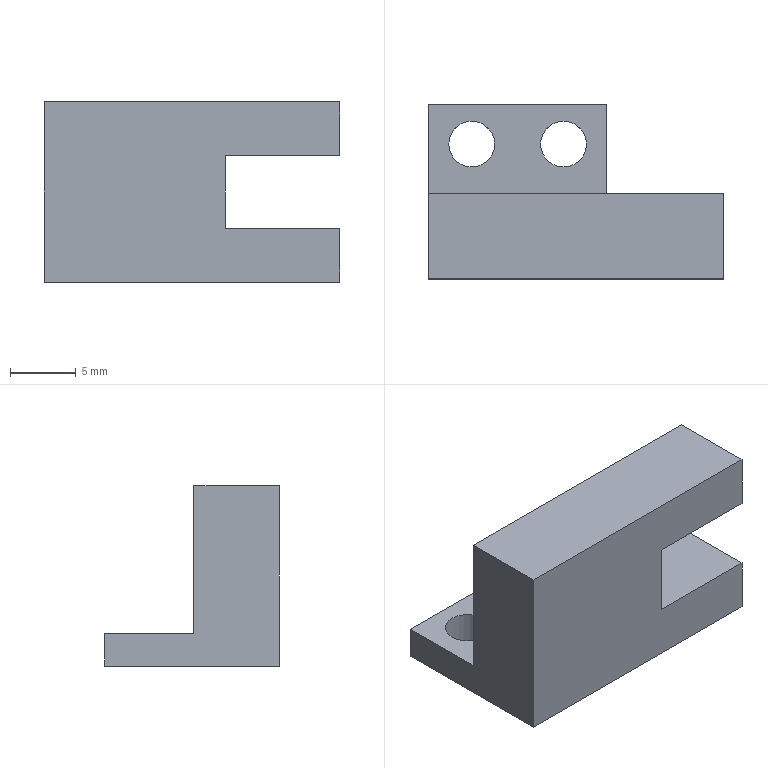Part | STEP file | PM-F54 | 1 solid | 17 faces | box 22.5 x 13.3 x 13.75 mm | volume 1880 mm3 | plane 13 | cylinder 4 | commonest cylinder face diameters 3.5 x4
STEP:
#1=CARTESIAN_POINT('',(5.05,10.3,2.5));
#2=VERTEX_POINT('',#1);
#3=CARTESIAN_POINT('',(1.55,10.3,2.5));
#4=VERTEX_POINT('',#3);
#5=CARTESIAN_POINT('',(3.3,10.3,2.5));
#6=DIRECTION('',(0.,0.,-1.));
#7=DIRECTION('',(-1.,0.,0.));
#8=AXIS2_PLACEMENT_3D('',#5,#6,#7);
#9=CIRCLE('',#8,1.75);
#10=EDGE_CURVE('',#2,#4,#9,.T.);
#11=ORIENTED_EDGE('',*,*,#10,.F.);
#12=CARTESIAN_POINT('',(5.05,10.3,0.));
#13=VERTEX_POINT('',#12);
#14=CARTESIAN_POINT('',(5.05,10.3,2.5));
#15=DIRECTION('',(0.,0.,-1.));
#16=VECTOR('',#15,1000.);
#17=LINE('',#14,#16);
#18=EDGE_CURVE('',#2,#13,#17,.T.);
#19=ORIENTED_EDGE('',*,*,#18,.T.);
#20=CARTESIAN_POINT('',(1.55,10.3,0.));
#21=VERTEX_POINT('',#20);
#22=CARTESIAN_POINT('',(3.3,10.3,0.));
#23=DIRECTION('',(0.,0.,-1.));
#24=DIRECTION('',(-1.,0.,0.));
#25=AXIS2_PLACEMENT_3D('',#22,#23,#24);
#26=CIRCLE('',#25,1.75);
#27=EDGE_CURVE('',#13,#21,#26,.T.);
#28=ORIENTED_EDGE('',*,*,#27,.T.);
#29=CARTESIAN_POINT('',(1.55,10.3,2.5));
#30=DIRECTION('',(0.,0.,-1.));
#31=VECTOR('',#30,1000.);
#32=LINE('',#29,#31);
#33=EDGE_CURVE('',#4,#21,#32,.T.);
#34=ORIENTED_EDGE('',*,*,#33,.F.);
#35=EDGE_LOOP('',(#11,#19,#28,#34));
#36=FACE_OUTER_BOUND('',#35,.T.);
#37=CARTESIAN_POINT('',(3.3,10.3,2.5));
#38=DIRECTION('',(0.,0.,-1.));
#39=DIRECTION('',(-1.,0.,0.));
#40=AXIS2_PLACEMENT_3D('',#37,#38,#39);
#41=CYLINDRICAL_SURFACE('',#40,1.75);
#42=ADVANCED_FACE('',(#36),#41,.F.);
#43=CARTESIAN_POINT('',(12.05,10.3,2.5));
#44=VERTEX_POINT('',#43);
#45=CARTESIAN_POINT('',(8.55,10.3,2.5));
#46=VERTEX_POINT('',#45);
#47=CARTESIAN_POINT('',(10.3,10.3,2.5));
#48=DIRECTION('',(0.,0.,-1.));
#49=DIRECTION('',(-1.,0.,0.));
#50=AXIS2_PLACEMENT_3D('',#47,#48,#49);
#51=CIRCLE('',#50,1.75);
#52=EDGE_CURVE('',#44,#46,#51,.T.);
#53=ORIENTED_EDGE('',*,*,#52,.F.);
#54=CARTESIAN_POINT('',(12.05,10.3,0.));
#55=VERTEX_POINT('',#54);
#56=CARTESIAN_POINT('',(12.05,10.3,2.5));
#57=DIRECTION('',(0.,0.,-1.));
#58=VECTOR('',#57,1000.);
#59=LINE('',#56,#58);
#60=EDGE_CURVE('',#44,#55,#59,.T.);
#61=ORIENTED_EDGE('',*,*,#60,.T.);
#62=CARTESIAN_POINT('',(8.55,10.3,0.));
#63=VERTEX_POINT('',#62);
#64=CARTESIAN_POINT('',(10.3,10.3,0.));
#65=DIRECTION('',(0.,0.,-1.));
#66=DIRECTION('',(-1.,0.,0.));
#67=AXIS2_PLACEMENT_3D('',#64,#65,#66);
#68=CIRCLE('',#67,1.75);
#69=EDGE_CURVE('',#55,#63,#68,.T.);
#70=ORIENTED_EDGE('',*,*,#69,.T.);
#71=CARTESIAN_POINT('',(8.55,10.3,2.5));
#72=DIRECTION('',(0.,0.,-1.));
#73=VECTOR('',#72,1000.);
#74=LINE('',#71,#73);
#75=EDGE_CURVE('',#46,#63,#74,.T.);
#76=ORIENTED_EDGE('',*,*,#75,.F.);
#77=EDGE_LOOP('',(#53,#61,#70,#76));
#78=FACE_OUTER_BOUND('',#77,.T.);
#79=CARTESIAN_POINT('',(10.3,10.3,2.5));
#80=DIRECTION('',(0.,0.,-1.));
#81=DIRECTION('',(-1.,0.,0.));
#82=AXIS2_PLACEMENT_3D('',#79,#80,#81);
#83=CYLINDRICAL_SURFACE('',#82,1.75);
#84=ADVANCED_FACE('',(#78),#83,.F.);
#85=CARTESIAN_POINT('',(13.6,6.5,2.5));
#86=VERTEX_POINT('',#85);
#87=CARTESIAN_POINT('',(13.6,6.5,0.));
#88=VERTEX_POINT('',#87);
#89=CARTESIAN_POINT('',(13.6,6.5,2.5));
#90=DIRECTION('',(0.,0.,-1.));
#91=VECTOR('',#90,1000.);
#92=LINE('',#89,#91);
#93=EDGE_CURVE('',#86,#88,#92,.T.);
#94=ORIENTED_EDGE('',*,*,#93,.F.);
#95=CARTESIAN_POINT('',(0.,6.5,2.5));
#96=VERTEX_POINT('',#95);
#97=CARTESIAN_POINT('',(0.,6.5,2.5));
#98=DIRECTION('',(-1.,0.,0.));
#99=VECTOR('',#98,1000.);
#100=LINE('',#97,#99);
#101=EDGE_CURVE('',#86,#96,#100,.T.);
#102=ORIENTED_EDGE('',*,*,#101,.T.);
#103=CARTESIAN_POINT('',(0.,6.5,13.75));
#104=VERTEX_POINT('',#103);
#105=CARTESIAN_POINT('',(0.,6.5,13.75));
#106=DIRECTION('',(0.,0.,-1.));
#107=VECTOR('',#106,1000.);
#108=LINE('',#105,#107);
#109=EDGE_CURVE('',#104,#96,#108,.T.);
#110=ORIENTED_EDGE('',*,*,#109,.F.);
#111=CARTESIAN_POINT('',(22.5,6.5,13.75));
#112=VERTEX_POINT('',#111);
#113=CARTESIAN_POINT('',(0.,6.5,13.75));
#114=DIRECTION('',(-1.,0.,0.));
#115=VECTOR('',#114,1000.);
#116=LINE('',#113,#115);
#117=EDGE_CURVE('',#112,#104,#116,.T.);
#118=ORIENTED_EDGE('',*,*,#117,.F.);
#119=CARTESIAN_POINT('',(22.5,6.5,9.65));
#120=VERTEX_POINT('',#119);
#121=CARTESIAN_POINT('',(22.5,6.5,13.75));
#122=DIRECTION('',(0.,0.,-1.));
#123=VECTOR('',#122,1000.);
#124=LINE('',#121,#123);
#125=EDGE_CURVE('',#112,#120,#124,.T.);
#126=ORIENTED_EDGE('',*,*,#125,.T.);
#127=CARTESIAN_POINT('',(13.8,6.5,9.65));
#128=VERTEX_POINT('',#127);
#129=CARTESIAN_POINT('',(0.,6.5,9.65));
#130=DIRECTION('',(-1.,0.,0.));
#131=VECTOR('',#130,1000.);
#132=LINE('',#129,#131);
#133=EDGE_CURVE('',#120,#128,#132,.T.);
#134=ORIENTED_EDGE('',*,*,#133,.T.);
#135=CARTESIAN_POINT('',(13.8,6.5,4.1));
#136=VERTEX_POINT('',#135);
#137=CARTESIAN_POINT('',(13.8,6.5,9.65));
#138=DIRECTION('',(0.,0.,-1.));
#139=VECTOR('',#138,1000.);
#140=LINE('',#137,#139);
#141=EDGE_CURVE('',#128,#136,#140,.T.);
#142=ORIENTED_EDGE('',*,*,#141,.T.);
#143=CARTESIAN_POINT('',(22.5,6.5,4.1));
#144=VERTEX_POINT('',#143);
#145=CARTESIAN_POINT('',(13.8,6.5,4.1));
#146=DIRECTION('',(1.,0.,0.));
#147=VECTOR('',#146,1000.);
#148=LINE('',#145,#147);
#149=EDGE_CURVE('',#136,#144,#148,.T.);
#150=ORIENTED_EDGE('',*,*,#149,.T.);
#151=CARTESIAN_POINT('',(22.5,6.5,0.));
#152=VERTEX_POINT('',#151);
#153=CARTESIAN_POINT('',(22.5,6.5,13.75));
#154=DIRECTION('',(0.,0.,-1.));
#155=VECTOR('',#154,1000.);
#156=LINE('',#153,#155);
#157=EDGE_CURVE('',#144,#152,#156,.T.);
#158=ORIENTED_EDGE('',*,*,#157,.T.);
#159=CARTESIAN_POINT('',(0.,6.5,0.));
#160=DIRECTION('',(-1.,0.,0.));
#161=VECTOR('',#160,1000.);
#162=LINE('',#159,#161);
#163=EDGE_CURVE('',#152,#88,#162,.T.);
#164=ORIENTED_EDGE('',*,*,#163,.T.);
#165=EDGE_LOOP('',(#94,#102,#110,#118,#126,#134,#142,#150,#158,#164));
#166=FACE_OUTER_BOUND('',#165,.T.);
#167=CARTESIAN_POINT('',(0.,6.5,13.75));
#168=DIRECTION('',(0.,-1.,0.));
#169=DIRECTION('',(0.,0.,-1.));
#170=AXIS2_PLACEMENT_3D('',#167,#168,#169);
#171=PLANE('',#170);
#172=ADVANCED_FACE('',(#166),#171,.F.);
#173=CARTESIAN_POINT('',(22.5,0.,13.75));
#174=VERTEX_POINT('',#173);
#175=CARTESIAN_POINT('',(22.5,0.,9.65));
#176=VERTEX_POINT('',#175);
#177=CARTESIAN_POINT('',(22.5,0.,13.75));
#178=DIRECTION('',(0.,0.,-1.));
#179=VECTOR('',#178,1000.);
#180=LINE('',#177,#179);
#181=EDGE_CURVE('',#174,#176,#180,.T.);
#182=ORIENTED_EDGE('',*,*,#181,.T.);
#183=CARTESIAN_POINT('',(22.5,0.,9.65));
#184=DIRECTION('',(0.,1.,0.));
#185=VECTOR('',#184,1000.);
#186=LINE('',#183,#185);
#187=EDGE_CURVE('',#176,#120,#186,.T.);
#188=ORIENTED_EDGE('',*,*,#187,.T.);
#189=ORIENTED_EDGE('',*,*,#125,.F.);
#190=CARTESIAN_POINT('',(22.5,0.,13.75));
#191=DIRECTION('',(0.,1.,0.));
#192=VECTOR('',#191,1000.);
#193=LINE('',#190,#192);
#194=EDGE_CURVE('',#174,#112,#193,.T.);
#195=ORIENTED_EDGE('',*,*,#194,.F.);
#196=EDGE_LOOP('',(#182,#188,#189,#195));
#197=FACE_OUTER_BOUND('',#196,.T.);
#198=CARTESIAN_POINT('',(22.5,0.,13.75));
#199=DIRECTION('',(-1.,0.,0.));
#200=DIRECTION('',(0.,0.,1.));
#201=AXIS2_PLACEMENT_3D('',#198,#199,#200);
#202=PLANE('',#201);
#203=ADVANCED_FACE('',(#197),#202,.F.);
#204=CARTESIAN_POINT('',(0.,13.3,0.));
#205=VERTEX_POINT('',#204);
#206=CARTESIAN_POINT('',(0.,0.,0.));
#207=VERTEX_POINT('',#206);
#208=CARTESIAN_POINT('',(0.,0.,0.));
#209=DIRECTION('',(0.,-1.,0.));
#210=VECTOR('',#209,1000.);
#211=LINE('',#208,#210);
#212=EDGE_CURVE('',#205,#207,#211,.T.);
#213=ORIENTED_EDGE('',*,*,#212,.T.);
#214=CARTESIAN_POINT('',(0.,0.,13.75));
#215=VERTEX_POINT('',#214);
#216=CARTESIAN_POINT('',(0.,0.,13.75));
#217=DIRECTION('',(0.,0.,-1.));
#218=VECTOR('',#217,1000.);
#219=LINE('',#216,#218);
#220=EDGE_CURVE('',#215,#207,#219,.T.);
#221=ORIENTED_EDGE('',*,*,#220,.F.);
#222=CARTESIAN_POINT('',(0.,0.,13.75));
#223=DIRECTION('',(0.,-1.,0.));
#224=VECTOR('',#223,1000.);
#225=LINE('',#222,#224);
#226=EDGE_CURVE('',#104,#215,#225,.T.);
#227=ORIENTED_EDGE('',*,*,#226,.F.);
#228=ORIENTED_EDGE('',*,*,#109,.T.);
#229=CARTESIAN_POINT('',(0.,13.3,2.5));
#230=VERTEX_POINT('',#229);
#231=CARTESIAN_POINT('',(0.,6.5,2.5));
#232=DIRECTION('',(0.,1.,0.));
#233=VECTOR('',#232,1000.);
#234=LINE('',#231,#233);
#235=EDGE_CURVE('',#96,#230,#234,.T.);
#236=ORIENTED_EDGE('',*,*,#235,.T.);
#237=CARTESIAN_POINT('',(0.,13.3,2.5));
#238=DIRECTION('',(0.,0.,-1.));
#239=VECTOR('',#238,1000.);
#240=LINE('',#237,#239);
#241=EDGE_CURVE('',#230,#205,#240,.T.);
#242=ORIENTED_EDGE('',*,*,#241,.T.);
#243=EDGE_LOOP('',(#213,#221,#227,#228,#236,#242));
#244=FACE_OUTER_BOUND('',#243,.T.);
#245=CARTESIAN_POINT('',(0.,0.,13.75));
#246=DIRECTION('',(1.,0.,0.));
#247=DIRECTION('',(0.,0.,-1.));
#248=AXIS2_PLACEMENT_3D('',#245,#246,#247);
#249=PLANE('',#248);
#250=ADVANCED_FACE('',(#244),#249,.F.);
#251=CARTESIAN_POINT('',(13.8,0.,9.65));
#252=VERTEX_POINT('',#251);
#253=CARTESIAN_POINT('',(13.8,0.,4.1));
#254=VERTEX_POINT('',#253);
#255=CARTESIAN_POINT('',(13.8,0.,9.65));
#256=DIRECTION('',(0.,0.,-1.));
#257=VECTOR('',#256,1000.);
#258=LINE('',#255,#257);
#259=EDGE_CURVE('',#252,#254,#258,.T.);
#260=ORIENTED_EDGE('',*,*,#259,.F.);
#261=CARTESIAN_POINT('',(13.8,0.,9.65));
#262=DIRECTION('',(-1.,0.,0.));
#263=VECTOR('',#262,1000.);
#264=LINE('',#261,#263);
#265=EDGE_CURVE('',#176,#252,#264,.T.);
#266=ORIENTED_EDGE('',*,*,#265,.F.);
#267=ORIENTED_EDGE('',*,*,#181,.F.);
#268=CARTESIAN_POINT('',(0.,0.,13.75));
#269=DIRECTION('',(1.,0.,0.));
#270=VECTOR('',#269,1000.);
#271=LINE('',#268,#270);
#272=EDGE_CURVE('',#215,#174,#271,.T.);
#273=ORIENTED_EDGE('',*,*,#272,.F.);
#274=ORIENTED_EDGE('',*,*,#220,.T.);
#275=CARTESIAN_POINT('',(22.5,0.,0.));
#276=VERTEX_POINT('',#275);
#277=CARTESIAN_POINT('',(0.,0.,0.));
#278=DIRECTION('',(1.,0.,0.));
#279=VECTOR('',#278,1000.);
#280=LINE('',#277,#279);
#281=EDGE_CURVE('',#207,#276,#280,.T.);
#282=ORIENTED_EDGE('',*,*,#281,.T.);
#283=CARTESIAN_POINT('',(22.5,0.,4.1));
#284=VERTEX_POINT('',#283);
#285=CARTESIAN_POINT('',(22.5,0.,13.75));
#286=DIRECTION('',(0.,0.,-1.));
#287=VECTOR('',#286,1000.);
#288=LINE('',#285,#287);
#289=EDGE_CURVE('',#284,#276,#288,.T.);
#290=ORIENTED_EDGE('',*,*,#289,.F.);
#291=CARTESIAN_POINT('',(13.8,0.,4.1));
#292=DIRECTION('',(1.,0.,0.));
#293=VECTOR('',#292,1000.);
#294=LINE('',#291,#293);
#295=EDGE_CURVE('',#254,#284,#294,.T.);
#296=ORIENTED_EDGE('',*,*,#295,.F.);
#297=EDGE_LOOP('',(#260,#266,#267,#273,#274,#282,#290,#296));
#298=FACE_OUTER_BOUND('',#297,.T.);
#299=CARTESIAN_POINT('',(0.,0.,13.75));
#300=DIRECTION('',(0.,1.,0.));
#301=DIRECTION('',(0.,0.,1.));
#302=AXIS2_PLACEMENT_3D('',#299,#300,#301);
#303=PLANE('',#302);
#304=ADVANCED_FACE('',(#298),#303,.F.);
#305=ORIENTED_EDGE('',*,*,#157,.F.);
#306=CARTESIAN_POINT('',(22.5,0.,4.1));
#307=DIRECTION('',(0.,-1.,0.));
#308=VECTOR('',#307,1000.);
#309=LINE('',#306,#308);
#310=EDGE_CURVE('',#144,#284,#309,.T.);
#311=ORIENTED_EDGE('',*,*,#310,.T.);
#312=ORIENTED_EDGE('',*,*,#289,.T.);
#313=CARTESIAN_POINT('',(22.5,0.,0.));
#314=DIRECTION('',(0.,1.,0.));
#315=VECTOR('',#314,1000.);
#316=LINE('',#313,#315);
#317=EDGE_CURVE('',#276,#152,#316,.T.);
#318=ORIENTED_EDGE('',*,*,#317,.T.);
#319=EDGE_LOOP('',(#305,#311,#312,#318));
#320=FACE_OUTER_BOUND('',#319,.T.);
#321=CARTESIAN_POINT('',(22.5,0.,13.75));
#322=DIRECTION('',(-1.,0.,0.));
#323=DIRECTION('',(0.,0.,1.));
#324=AXIS2_PLACEMENT_3D('',#321,#322,#323);
#325=PLANE('',#324);
#326=ADVANCED_FACE('',(#320),#325,.F.);
#327=ORIENTED_EDGE('',*,*,#226,.T.);
#328=ORIENTED_EDGE('',*,*,#272,.T.);
#329=ORIENTED_EDGE('',*,*,#194,.T.);
#330=ORIENTED_EDGE('',*,*,#117,.T.);
#331=EDGE_LOOP('',(#327,#328,#329,#330));
#332=FACE_OUTER_BOUND('',#331,.T.);
#333=CARTESIAN_POINT('',(0.,6.5,13.75));
#334=DIRECTION('',(0.,0.,-1.));
#335=DIRECTION('',(-1.,0.,0.));
#336=AXIS2_PLACEMENT_3D('',#333,#334,#335);
#337=PLANE('',#336);
#338=ADVANCED_FACE('',(#332),#337,.F.);
#339=ORIENTED_EDGE('',*,*,#212,.F.);
#340=CARTESIAN_POINT('',(13.6,13.3,0.));
#341=VERTEX_POINT('',#340);
#342=CARTESIAN_POINT('',(0.,13.3,0.));
#343=DIRECTION('',(1.,0.,0.));
#344=VECTOR('',#343,1000.);
#345=LINE('',#342,#344);
#346=EDGE_CURVE('',#205,#341,#345,.T.);
#347=ORIENTED_EDGE('',*,*,#346,.T.);
#348=CARTESIAN_POINT('',(13.6,6.5,0.));
#349=DIRECTION('',(0.,-1.,0.));
#350=VECTOR('',#349,1000.);
#351=LINE('',#348,#350);
#352=EDGE_CURVE('',#341,#88,#351,.T.);
#353=ORIENTED_EDGE('',*,*,#352,.T.);
#354=ORIENTED_EDGE('',*,*,#163,.F.);
#355=ORIENTED_EDGE('',*,*,#317,.F.);
#356=ORIENTED_EDGE('',*,*,#281,.F.);
#357=EDGE_LOOP('',(#339,#347,#353,#354,#355,#356));
#358=FACE_OUTER_BOUND('',#357,.T.);
#359=CARTESIAN_POINT('',(3.3,10.3,0.));
#360=DIRECTION('',(0.,0.,-1.));
#361=DIRECTION('',(-1.,0.,0.));
#362=AXIS2_PLACEMENT_3D('',#359,#360,#361);
#363=CIRCLE('',#362,1.75);
#364=EDGE_CURVE('',#21,#13,#363,.T.);
#365=ORIENTED_EDGE('',*,*,#364,.F.);
#366=ORIENTED_EDGE('',*,*,#27,.F.);
#367=EDGE_LOOP('',(#365,#366));
#368=FACE_BOUND('',#367,.T.);
#369=CARTESIAN_POINT('',(10.3,10.3,0.));
#370=DIRECTION('',(0.,0.,-1.));
#371=DIRECTION('',(-1.,0.,0.));
#372=AXIS2_PLACEMENT_3D('',#369,#370,#371);
#373=CIRCLE('',#372,1.75);
#374=EDGE_CURVE('',#63,#55,#373,.T.);
#375=ORIENTED_EDGE('',*,*,#374,.F.);
#376=ORIENTED_EDGE('',*,*,#69,.F.);
#377=EDGE_LOOP('',(#375,#376));
#378=FACE_BOUND('',#377,.T.);
#379=CARTESIAN_POINT('',(0.,6.5,0.));
#380=DIRECTION('',(0.,0.,-1.));
#381=DIRECTION('',(-1.,0.,0.));
#382=AXIS2_PLACEMENT_3D('',#379,#380,#381);
#383=PLANE('',#382);
#384=ADVANCED_FACE('',(#358,#368,#378),#383,.T.);
#385=ORIENTED_EDGE('',*,*,#265,.T.);
#386=CARTESIAN_POINT('',(13.8,6.5,9.65));
#387=DIRECTION('',(0.,-1.,0.));
#388=VECTOR('',#387,1000.);
#389=LINE('',#386,#388);
#390=EDGE_CURVE('',#128,#252,#389,.T.);
#391=ORIENTED_EDGE('',*,*,#390,.F.);
#392=ORIENTED_EDGE('',*,*,#133,.F.);
#393=ORIENTED_EDGE('',*,*,#187,.F.);
#394=EDGE_LOOP('',(#385,#391,#392,#393));
#395=FACE_OUTER_BOUND('',#394,.T.);
#396=CARTESIAN_POINT('',(13.8,6.5,9.65));
#397=DIRECTION('',(0.,0.,1.));
#398=DIRECTION('',(1.,0.,0.));
#399=AXIS2_PLACEMENT_3D('',#396,#397,#398);
#400=PLANE('',#399);
#401=ADVANCED_FACE('',(#395),#400,.F.);
#402=ORIENTED_EDGE('',*,*,#149,.F.);
#403=CARTESIAN_POINT('',(13.8,6.5,4.1));
#404=DIRECTION('',(0.,-1.,0.));
#405=VECTOR('',#404,1000.);
#406=LINE('',#403,#405);
#407=EDGE_CURVE('',#136,#254,#406,.T.);
#408=ORIENTED_EDGE('',*,*,#407,.T.);
#409=ORIENTED_EDGE('',*,*,#295,.T.);
#410=ORIENTED_EDGE('',*,*,#310,.F.);
#411=EDGE_LOOP('',(#402,#408,#409,#410));
#412=FACE_OUTER_BOUND('',#411,.T.);
#413=CARTESIAN_POINT('',(13.8,6.5,4.1));
#414=DIRECTION('',(0.,0.,-1.));
#415=DIRECTION('',(-1.,0.,0.));
#416=AXIS2_PLACEMENT_3D('',#413,#414,#415);
#417=PLANE('',#416);
#418=ADVANCED_FACE('',(#412),#417,.F.);
#419=ORIENTED_EDGE('',*,*,#259,.T.);
#420=ORIENTED_EDGE('',*,*,#407,.F.);
#421=ORIENTED_EDGE('',*,*,#141,.F.);
#422=ORIENTED_EDGE('',*,*,#390,.T.);
#423=EDGE_LOOP('',(#419,#420,#421,#422));
#424=FACE_OUTER_BOUND('',#423,.T.);
#425=CARTESIAN_POINT('',(13.8,6.5,9.65));
#426=DIRECTION('',(-1.,0.,0.));
#427=DIRECTION('',(0.,0.,1.));
#428=AXIS2_PLACEMENT_3D('',#425,#426,#427);
#429=PLANE('',#428);
#430=ADVANCED_FACE('',(#424),#429,.F.);
#431=ORIENTED_EDGE('',*,*,#352,.F.);
#432=CARTESIAN_POINT('',(13.6,13.3,2.5));
#433=VERTEX_POINT('',#432);
#434=CARTESIAN_POINT('',(13.6,13.3,2.5));
#435=DIRECTION('',(0.,0.,-1.));
#436=VECTOR('',#435,1000.);
#437=LINE('',#434,#436);
#438=EDGE_CURVE('',#433,#341,#437,.T.);
#439=ORIENTED_EDGE('',*,*,#438,.F.);
#440=CARTESIAN_POINT('',(13.6,6.5,2.5));
#441=DIRECTION('',(0.,-1.,0.));
#442=VECTOR('',#441,1000.);
#443=LINE('',#440,#442);
#444=EDGE_CURVE('',#433,#86,#443,.T.);
#445=ORIENTED_EDGE('',*,*,#444,.T.);
#446=ORIENTED_EDGE('',*,*,#93,.T.);
#447=EDGE_LOOP('',(#431,#439,#445,#446));
#448=FACE_OUTER_BOUND('',#447,.T.);
#449=CARTESIAN_POINT('',(13.6,6.5,2.5));
#450=DIRECTION('',(1.,0.,0.));
#451=DIRECTION('',(0.,0.,-1.));
#452=AXIS2_PLACEMENT_3D('',#449,#450,#451);
#453=PLANE('',#452);
#454=ADVANCED_FACE('',(#448),#453,.T.);
#455=ORIENTED_EDGE('',*,*,#346,.F.);
#456=ORIENTED_EDGE('',*,*,#241,.F.);
#457=CARTESIAN_POINT('',(0.,13.3,2.5));
#458=DIRECTION('',(1.,0.,0.));
#459=VECTOR('',#458,1000.);
#460=LINE('',#457,#459);
#461=EDGE_CURVE('',#230,#433,#460,.T.);
#462=ORIENTED_EDGE('',*,*,#461,.T.);
#463=ORIENTED_EDGE('',*,*,#438,.T.);
#464=EDGE_LOOP('',(#455,#456,#462,#463));
#465=FACE_OUTER_BOUND('',#464,.T.);
#466=CARTESIAN_POINT('',(0.,13.3,2.5));
#467=DIRECTION('',(0.,1.,0.));
#468=DIRECTION('',(-1.,0.,0.));
#469=AXIS2_PLACEMENT_3D('',#466,#467,#468);
#470=PLANE('',#469);
#471=ADVANCED_FACE('',(#465),#470,.T.);
#472=CARTESIAN_POINT('',(3.3,10.3,2.5));
#473=DIRECTION('',(0.,0.,-1.));
#474=DIRECTION('',(-1.,0.,0.));
#475=AXIS2_PLACEMENT_3D('',#472,#473,#474);
#476=CIRCLE('',#475,1.75);
#477=EDGE_CURVE('',#4,#2,#476,.T.);
#478=ORIENTED_EDGE('',*,*,#477,.T.);
#479=ORIENTED_EDGE('',*,*,#10,.T.);
#480=EDGE_LOOP('',(#478,#479));
#481=FACE_BOUND('',#480,.T.);
#482=CARTESIAN_POINT('',(10.3,10.3,2.5));
#483=DIRECTION('',(0.,0.,-1.));
#484=DIRECTION('',(-1.,0.,0.));
#485=AXIS2_PLACEMENT_3D('',#482,#483,#484);
#486=CIRCLE('',#485,1.75);
#487=EDGE_CURVE('',#46,#44,#486,.T.);
#488=ORIENTED_EDGE('',*,*,#487,.T.);
#489=ORIENTED_EDGE('',*,*,#52,.T.);
#490=EDGE_LOOP('',(#488,#489));
#491=FACE_BOUND('',#490,.T.);
#492=ORIENTED_EDGE('',*,*,#235,.F.);
#493=ORIENTED_EDGE('',*,*,#101,.F.);
#494=ORIENTED_EDGE('',*,*,#444,.F.);
#495=ORIENTED_EDGE('',*,*,#461,.F.);
#496=EDGE_LOOP('',(#492,#493,#494,#495));
#497=FACE_OUTER_BOUND('',#496,.T.);
#498=CARTESIAN_POINT('',(0.,13.3,2.5));
#499=DIRECTION('',(0.,0.,-1.));
#500=DIRECTION('',(-1.,0.,0.));
#501=AXIS2_PLACEMENT_3D('',#498,#499,#500);
#502=PLANE('',#501);
#503=ADVANCED_FACE('',(#481,#491,#497),#502,.F.);
#504=ORIENTED_EDGE('',*,*,#60,.F.);
#505=ORIENTED_EDGE('',*,*,#487,.F.);
#506=ORIENTED_EDGE('',*,*,#75,.T.);
#507=ORIENTED_EDGE('',*,*,#374,.T.);
#508=EDGE_LOOP('',(#504,#505,#506,#507));
#509=FACE_OUTER_BOUND('',#508,.T.);
#510=CARTESIAN_POINT('',(10.3,10.3,2.5));
#511=DIRECTION('',(0.,0.,-1.));
#512=DIRECTION('',(-1.,0.,0.));
#513=AXIS2_PLACEMENT_3D('',#510,#511,#512);
#514=CYLINDRICAL_SURFACE('',#513,1.75);
#515=ADVANCED_FACE('',(#509),#514,.F.);
#516=ORIENTED_EDGE('',*,*,#18,.F.);
#517=ORIENTED_EDGE('',*,*,#477,.F.);
#518=ORIENTED_EDGE('',*,*,#33,.T.);
#519=ORIENTED_EDGE('',*,*,#364,.T.);
#520=EDGE_LOOP('',(#516,#517,#518,#519));
#521=FACE_OUTER_BOUND('',#520,.T.);
#522=CARTESIAN_POINT('',(3.3,10.3,2.5));
#523=DIRECTION('',(0.,0.,-1.));
#524=DIRECTION('',(-1.,0.,0.));
#525=AXIS2_PLACEMENT_3D('',#522,#523,#524);
#526=CYLINDRICAL_SURFACE('',#525,1.75);
#527=ADVANCED_FACE('',(#521),#526,.F.);
#528=CLOSED_SHELL('',(#42,#84,#172,#203,#250,#304,#326,#338,#384,#401,#418,#430,#454,#471,#503,#515,#527));
#529=MANIFOLD_SOLID_BREP('',#528);
#530=CARTESIAN_POINT('',(0.,0.,0.));
#531=DIRECTION('',(0.,0.,1.));
#532=DIRECTION('',(1.,0.,0.));
#533=AXIS2_PLACEMENT_3D('',#530,#531,#532);
#534=(LENGTH_UNIT()NAMED_UNIT(*)SI_UNIT(.MILLI.,.METRE.));
#535=UNCERTAINTY_MEASURE_WITH_UNIT(LENGTH_MEASURE(0.00001),#534,'','');
#536=(NAMED_UNIT(*)PLANE_ANGLE_UNIT()SI_UNIT($,.RADIAN.));
#537=(NAMED_UNIT(*)SI_UNIT($,.STERADIAN.)SOLID_ANGLE_UNIT());
#538=(GEOMETRIC_REPRESENTATION_CONTEXT(3)GLOBAL_UNCERTAINTY_ASSIGNED_CONTEXT((#535))GLOBAL_UNIT_ASSIGNED_CONTEXT((#534,#536,#537))REPRESENTATION_CONTEXT('',''));
#539=ADVANCED_BREP_SHAPE_REPRESENTATION('',(#529,#533),#538);